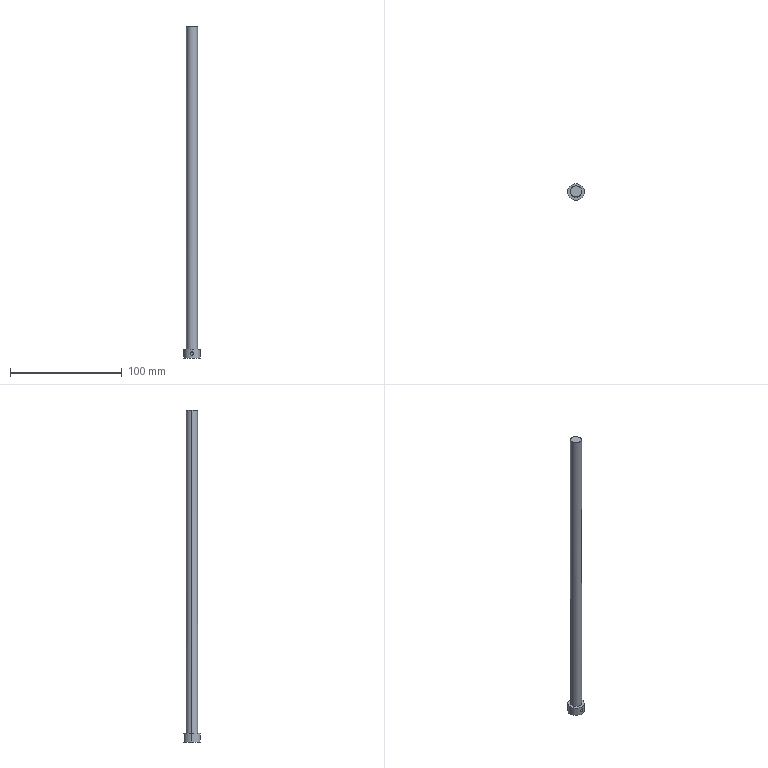Part | Creo | 1 solid | 10 faces | box 15 x 15 x 297.5 mm | volume 24082 mm3 | cylinder 6 | plane 4 | commonest cylinder face diameters 3 x2 10 x2 15 x2
STEP:
#1=CARTESIAN_POINT('',(-40.,-141.,-252.5));
#2=VERTEX_POINT('',#1);
#3=CARTESIAN_POINT('',(-50.,-141.,-252.5));
#4=VERTEX_POINT('',#3);
#5=CARTESIAN_POINT('',(-45.,-141.,-252.5));
#6=DIRECTION('',(0.,0.,-1.));
#7=DIRECTION('',(1.,0.,0.));
#8=AXIS2_PLACEMENT_3D('',#5,#6,#7);
#9=CIRCLE('',#8,5.);
#10=EDGE_CURVE('',#2,#4,#9,.T.);
#11=ORIENTED_EDGE('',*,*,#10,.T.);
#12=CARTESIAN_POINT('',(-50.,-141.,37.));
#13=VERTEX_POINT('',#12);
#14=CARTESIAN_POINT('',(-50.,-141.,37.));
#15=DIRECTION('',(0.,0.,-1.));
#16=VECTOR('',#15,289.5);
#17=LINE('',#14,#16);
#18=EDGE_CURVE('',#13,#4,#17,.T.);
#19=ORIENTED_EDGE('',*,*,#18,.F.);
#20=CARTESIAN_POINT('',(-40.,-141.,36.619));
#21=VERTEX_POINT('',#20);
#22=CARTESIAN_POINT('',(-50.,-141.,37.));
#23=CARTESIAN_POINT('',(-50.,-141.589,37.));
#24=CARTESIAN_POINT('',(-49.785,-142.862,36.992));
#25=CARTESIAN_POINT('',(-48.645,-144.641,36.949));
#26=CARTESIAN_POINT('',(-46.85,-145.786,36.88));
#27=CARTESIAN_POINT('',(-45.,-146.107,36.809));
#28=CARTESIAN_POINT('',(-43.15,-145.786,36.739));
#29=CARTESIAN_POINT('',(-41.355,-144.641,36.67));
#30=CARTESIAN_POINT('',(-40.215,-142.862,36.627));
#31=CARTESIAN_POINT('',(-40.,-141.589,36.619));
#32=CARTESIAN_POINT('',(-40.,-141.,36.619));
#33=B_SPLINE_CURVE_WITH_KNOTS('',3,(#22,#23,#24,#25,#26,#27,#28,#29,#30,#31,#32),.UNSPECIFIED.,.F.,.F.,(4,1,1,1,1,1,1,1,4),(0.,0.125,0.25,0.375,0.5,0.625,0.75,0.875,1.),.UNSPECIFIED.);
#34=EDGE_CURVE('',#13,#21,#33,.T.);
#35=ORIENTED_EDGE('',*,*,#34,.T.);
#36=CARTESIAN_POINT('',(-40.,-141.,36.619));
#37=DIRECTION('',(0.,0.,-1.));
#38=VECTOR('',#37,289.119);
#39=LINE('',#36,#38);
#40=EDGE_CURVE('',#21,#2,#39,.T.);
#41=ORIENTED_EDGE('',*,*,#40,.T.);
#42=EDGE_LOOP('',(#11,#19,#35,#41));
#43=FACE_OUTER_BOUND('',#42,.F.);
#44=CARTESIAN_POINT('',(-45.,-141.,135.));
#45=DIRECTION('',(0.,0.,-1.));
#46=DIRECTION('',(1.,0.,0.));
#47=AXIS2_PLACEMENT_3D('',#44,#45,#46);
#48=CYLINDRICAL_SURFACE('',#47,5.);
#49=ADVANCED_FACE('',(#43),#48,.T.);
#50=CARTESIAN_POINT('',(-52.5,-141.,-252.5));
#51=VERTEX_POINT('',#50);
#52=CARTESIAN_POINT('',(-37.5,-141.,-252.5));
#53=VERTEX_POINT('',#52);
#54=CARTESIAN_POINT('',(-45.,-141.,-252.5));
#55=DIRECTION('',(0.,0.,1.));
#56=DIRECTION('',(-1.,0.,0.));
#57=AXIS2_PLACEMENT_3D('',#54,#55,#56);
#58=CIRCLE('',#57,7.5);
#59=EDGE_CURVE('',#51,#53,#58,.T.);
#60=ORIENTED_EDGE('',*,*,#59,.F.);
#61=CARTESIAN_POINT('',(-45.,-141.,-252.5));
#62=DIRECTION('',(0.,0.,1.));
#63=DIRECTION('',(1.,0.,0.));
#64=AXIS2_PLACEMENT_3D('',#61,#62,#63);
#65=CIRCLE('',#64,7.5);
#66=EDGE_CURVE('',#53,#51,#65,.T.);
#67=ORIENTED_EDGE('',*,*,#66,.F.);
#68=EDGE_LOOP('',(#60,#67));
#69=FACE_OUTER_BOUND('',#68,.F.);
#70=CARTESIAN_POINT('',(-45.,-141.,-252.5));
#71=DIRECTION('',(0.,0.,-1.));
#72=DIRECTION('',(-1.,0.,0.));
#73=AXIS2_PLACEMENT_3D('',#70,#71,#72);
#74=CIRCLE('',#73,5.);
#75=EDGE_CURVE('',#4,#2,#74,.T.);
#76=ORIENTED_EDGE('',*,*,#75,.F.);
#77=ORIENTED_EDGE('',*,*,#10,.F.);
#78=EDGE_LOOP('',(#76,#77));
#79=FACE_BOUND('',#78,.F.);
#80=CARTESIAN_POINT('',(-45.,-141.,-252.5));
#81=DIRECTION('',(0.,0.,1.));
#82=DIRECTION('',(-1.,0.,0.));
#83=AXIS2_PLACEMENT_3D('',#80,#81,#82);
#84=PLANE('',#83);
#85=ADVANCED_FACE('',(#69,#79),#84,.T.);
#86=ORIENTED_EDGE('',*,*,#75,.T.);
#87=ORIENTED_EDGE('',*,*,#40,.F.);
#88=CARTESIAN_POINT('',(-40.,-141.,36.619));
#89=CARTESIAN_POINT('',(-40.,-140.411,36.619));
#90=CARTESIAN_POINT('',(-40.215,-139.138,36.627));
#91=CARTESIAN_POINT('',(-41.355,-137.359,36.67));
#92=CARTESIAN_POINT('',(-43.15,-136.214,36.739));
#93=CARTESIAN_POINT('',(-45.,-135.893,36.809));
#94=CARTESIAN_POINT('',(-46.85,-136.214,36.88));
#95=CARTESIAN_POINT('',(-48.645,-137.359,36.949));
#96=CARTESIAN_POINT('',(-49.785,-139.138,36.992));
#97=CARTESIAN_POINT('',(-50.,-140.411,37.));
#98=CARTESIAN_POINT('',(-50.,-141.,37.));
#99=B_SPLINE_CURVE_WITH_KNOTS('',3,(#88,#89,#90,#91,#92,#93,#94,#95,#96,#97,#98),.UNSPECIFIED.,.F.,.F.,(4,1,1,1,1,1,1,1,4),(0.,0.125,0.25,0.375,0.5,0.625,0.75,0.875,1.),.UNSPECIFIED.);
#100=EDGE_CURVE('',#21,#13,#99,.T.);
#101=ORIENTED_EDGE('',*,*,#100,.T.);
#102=ORIENTED_EDGE('',*,*,#18,.T.);
#103=EDGE_LOOP('',(#86,#87,#101,#102));
#104=FACE_OUTER_BOUND('',#103,.F.);
#105=CARTESIAN_POINT('',(-45.,-141.,135.));
#106=DIRECTION('',(0.,0.,-1.));
#107=DIRECTION('',(1.,0.,0.));
#108=AXIS2_PLACEMENT_3D('',#105,#106,#107);
#109=CYLINDRICAL_SURFACE('',#108,5.);
#110=ADVANCED_FACE('',(#104),#109,.T.);
#111=ORIENTED_EDGE('',*,*,#100,.F.);
#112=ORIENTED_EDGE('',*,*,#34,.F.);
#113=EDGE_LOOP('',(#111,#112));
#114=FACE_OUTER_BOUND('',#113,.F.);
#115=CARTESIAN_POINT('',(0.9569,31.474,35.055));
#116=DIRECTION('',(0.03814,0.,0.9993));
#117=DIRECTION('',(0.9993,0.,-0.03814));
#118=AXIS2_PLACEMENT_3D('',#115,#116,#117);
#119=PLANE('',#118);
#120=ADVANCED_FACE('',(#114),#119,.T.);
#121=ORIENTED_EDGE('',*,*,#59,.T.);
#122=CARTESIAN_POINT('',(-37.5,-141.,-260.5));
#123=VERTEX_POINT('',#122);
#124=CARTESIAN_POINT('',(-37.5,-141.,-260.5));
#125=DIRECTION('',(0.,0.,1.));
#126=VECTOR('',#125,8.);
#127=LINE('',#124,#126);
#128=EDGE_CURVE('',#123,#53,#127,.T.);
#129=ORIENTED_EDGE('',*,*,#128,.F.);
#130=CARTESIAN_POINT('',(-52.5,-141.,-260.5));
#131=VERTEX_POINT('',#130);
#132=CARTESIAN_POINT('',(-45.,-141.,-260.5));
#133=DIRECTION('',(0.,0.,-1.));
#134=DIRECTION('',(1.,0.,0.));
#135=AXIS2_PLACEMENT_3D('',#132,#133,#134);
#136=CIRCLE('',#135,7.5);
#137=EDGE_CURVE('',#123,#131,#136,.T.);
#138=ORIENTED_EDGE('',*,*,#137,.T.);
#139=CARTESIAN_POINT('',(-52.5,-141.,-260.5));
#140=DIRECTION('',(0.,0.,1.));
#141=VECTOR('',#140,8.);
#142=LINE('',#139,#141);
#143=EDGE_CURVE('',#131,#51,#142,.T.);
#144=ORIENTED_EDGE('',*,*,#143,.T.);
#145=EDGE_LOOP('',(#121,#129,#138,#144));
#146=FACE_OUTER_BOUND('',#145,.F.);
#147=CARTESIAN_POINT('',(-45.,-148.5,-258.));
#148=VERTEX_POINT('',#147);
#149=CARTESIAN_POINT('',(-45.,-148.5,-255.));
#150=VERTEX_POINT('',#149);
#151=CARTESIAN_POINT('',(-45.,-148.5,-258.));
#152=CARTESIAN_POINT('',(-45.205,-148.5,-258.));
#153=CARTESIAN_POINT('',(-45.583,-148.484,-257.922));
#154=CARTESIAN_POINT('',(-46.09,-148.425,-257.589));
#155=CARTESIAN_POINT('',(-46.424,-148.365,-257.085));
#156=CARTESIAN_POINT('',(-46.539,-148.34,-256.497));
#157=CARTESIAN_POINT('',(-46.422,-148.365,-255.912));
#158=CARTESIAN_POINT('',(-46.091,-148.425,-255.413));
#159=CARTESIAN_POINT('',(-45.585,-148.484,-255.078));
#160=CARTESIAN_POINT('',(-45.206,-148.5,-255.));
#161=CARTESIAN_POINT('',(-45.,-148.5,-255.));
#162=B_SPLINE_CURVE_WITH_KNOTS('',3,(#151,#152,#153,#154,#155,#156,#157,#158,#159,#160,#161),.UNSPECIFIED.,.F.,.F.,(4,1,1,1,1,1,1,1,4),(0.,0.125,0.25,0.375,0.5,0.625,0.75,0.875,1.),.UNSPECIFIED.);
#163=EDGE_CURVE('',#148,#150,#162,.T.);
#164=ORIENTED_EDGE('',*,*,#163,.F.);
#165=CARTESIAN_POINT('',(-45.,-148.5,-255.));
#166=CARTESIAN_POINT('',(-44.794,-148.5,-255.));
#167=CARTESIAN_POINT('',(-44.415,-148.484,-255.078));
#168=CARTESIAN_POINT('',(-43.907,-148.424,-255.414));
#169=CARTESIAN_POINT('',(-43.576,-148.364,-255.917));
#170=CARTESIAN_POINT('',(-43.461,-148.34,-256.506));
#171=CARTESIAN_POINT('',(-43.579,-148.365,-257.089));
#172=CARTESIAN_POINT('',(-43.908,-148.424,-257.586));
#173=CARTESIAN_POINT('',(-44.414,-148.484,-257.922));
#174=CARTESIAN_POINT('',(-44.794,-148.5,-258.));
#175=CARTESIAN_POINT('',(-45.,-148.5,-258.));
#176=B_SPLINE_CURVE_WITH_KNOTS('',3,(#165,#166,#167,#168,#169,#170,#171,#172,#173,#174,#175),.UNSPECIFIED.,.F.,.F.,(4,1,1,1,1,1,1,1,4),(0.,0.125,0.25,0.375,0.5,0.625,0.75,0.875,1.),.UNSPECIFIED.);
#177=EDGE_CURVE('',#150,#148,#176,.T.);
#178=ORIENTED_EDGE('',*,*,#177,.F.);
#179=EDGE_LOOP('',(#164,#178));
#180=FACE_BOUND('',#179,.F.);
#181=CARTESIAN_POINT('',(-45.,-141.,-260.5));
#182=DIRECTION('',(0.,0.,1.));
#183=DIRECTION('',(-1.,0.,0.));
#184=AXIS2_PLACEMENT_3D('',#181,#182,#183);
#185=CYLINDRICAL_SURFACE('',#184,7.5);
#186=ADVANCED_FACE('',(#146,#180),#185,.T.);
#187=ORIENTED_EDGE('',*,*,#163,.T.);
#188=CARTESIAN_POINT('',(-45.,-141.,-255.));
#189=VERTEX_POINT('',#188);
#190=CARTESIAN_POINT('',(-45.,-141.,-255.));
#191=DIRECTION('',(0.000000004,-1.,-0.000006083));
#192=VECTOR('',#191,7.5);
#193=LINE('',#190,#192);
#194=EDGE_CURVE('',#189,#150,#193,.T.);
#195=ORIENTED_EDGE('',*,*,#194,.F.);
#196=CARTESIAN_POINT('',(-45.,-141.,-258.));
#197=VERTEX_POINT('',#196);
#198=CARTESIAN_POINT('',(-45.,-141.,-256.5));
#199=DIRECTION('',(0.,-1.,0.));
#200=DIRECTION('',(0.,0.,1.));
#201=AXIS2_PLACEMENT_3D('',#198,#199,#200);
#202=CIRCLE('',#201,1.5);
#203=EDGE_CURVE('',#189,#197,#202,.T.);
#204=ORIENTED_EDGE('',*,*,#203,.T.);
#205=CARTESIAN_POINT('',(-45.,-141.,-258.));
#206=DIRECTION('',(0.,-1.,0.));
#207=VECTOR('',#206,7.5);
#208=LINE('',#205,#207);
#209=EDGE_CURVE('',#197,#148,#208,.T.);
#210=ORIENTED_EDGE('',*,*,#209,.T.);
#211=EDGE_LOOP('',(#187,#195,#204,#210));
#212=FACE_OUTER_BOUND('',#211,.F.);
#213=CARTESIAN_POINT('',(-45.,-141.,-256.5));
#214=DIRECTION('',(0.,-1.,0.));
#215=DIRECTION('',(0.,0.,-1.));
#216=AXIS2_PLACEMENT_3D('',#213,#214,#215);
#217=CYLINDRICAL_SURFACE('',#216,1.5);
#218=ADVANCED_FACE('',(#212),#217,.F.);
#219=ORIENTED_EDGE('',*,*,#177,.T.);
#220=ORIENTED_EDGE('',*,*,#209,.F.);
#221=CARTESIAN_POINT('',(-45.,-141.,-256.5));
#222=DIRECTION('',(0.,-1.,0.));
#223=DIRECTION('',(0.,0.,-1.));
#224=AXIS2_PLACEMENT_3D('',#221,#222,#223);
#225=CIRCLE('',#224,1.5);
#226=EDGE_CURVE('',#197,#189,#225,.T.);
#227=ORIENTED_EDGE('',*,*,#226,.T.);
#228=ORIENTED_EDGE('',*,*,#194,.T.);
#229=EDGE_LOOP('',(#219,#220,#227,#228));
#230=FACE_OUTER_BOUND('',#229,.F.);
#231=CARTESIAN_POINT('',(-45.,-141.,-256.5));
#232=DIRECTION('',(0.,-1.,0.));
#233=DIRECTION('',(0.,0.,-1.));
#234=AXIS2_PLACEMENT_3D('',#231,#232,#233);
#235=CYLINDRICAL_SURFACE('',#234,1.5);
#236=ADVANCED_FACE('',(#230),#235,.F.);
#237=ORIENTED_EDGE('',*,*,#226,.F.);
#238=ORIENTED_EDGE('',*,*,#203,.F.);
#239=EDGE_LOOP('',(#237,#238));
#240=FACE_OUTER_BOUND('',#239,.F.);
#241=CARTESIAN_POINT('',(-45.,-141.,-256.5));
#242=DIRECTION('',(0.,1.,0.));
#243=DIRECTION('',(0.,0.,1.));
#244=AXIS2_PLACEMENT_3D('',#241,#242,#243);
#245=PLANE('',#244);
#246=ADVANCED_FACE('',(#240),#245,.F.);
#247=ORIENTED_EDGE('',*,*,#66,.T.);
#248=ORIENTED_EDGE('',*,*,#143,.F.);
#249=CARTESIAN_POINT('',(-45.,-141.,-260.5));
#250=DIRECTION('',(0.,0.,-1.));
#251=DIRECTION('',(-1.,0.,0.));
#252=AXIS2_PLACEMENT_3D('',#249,#250,#251);
#253=CIRCLE('',#252,7.5);
#254=EDGE_CURVE('',#131,#123,#253,.T.);
#255=ORIENTED_EDGE('',*,*,#254,.T.);
#256=ORIENTED_EDGE('',*,*,#128,.T.);
#257=EDGE_LOOP('',(#247,#248,#255,#256));
#258=FACE_OUTER_BOUND('',#257,.F.);
#259=CARTESIAN_POINT('',(-45.,-141.,-260.5));
#260=DIRECTION('',(0.,0.,1.));
#261=DIRECTION('',(-1.,0.,0.));
#262=AXIS2_PLACEMENT_3D('',#259,#260,#261);
#263=CYLINDRICAL_SURFACE('',#262,7.5);
#264=ADVANCED_FACE('',(#258),#263,.T.);
#265=ORIENTED_EDGE('',*,*,#137,.F.);
#266=ORIENTED_EDGE('',*,*,#254,.F.);
#267=EDGE_LOOP('',(#265,#266));
#268=FACE_OUTER_BOUND('',#267,.F.);
#269=CARTESIAN_POINT('',(217.714,1.015,-260.5));
#270=DIRECTION('',(0.,0.,-1.));
#271=DIRECTION('',(1.,0.,0.));
#272=AXIS2_PLACEMENT_3D('',#269,#270,#271);
#273=PLANE('',#272);
#274=ADVANCED_FACE('',(#268),#273,.T.);
#275=CLOSED_SHELL('',(#49,#85,#110,#120,#186,#218,#236,#246,#264,#274));
#276=MANIFOLD_SOLID_BREP('',#275);
#277=(LENGTH_UNIT()NAMED_UNIT(*)SI_UNIT(.MILLI.,.METRE.));
#278=UNCERTAINTY_MEASURE_WITH_UNIT(LENGTH_MEASURE(0.02982),#277,'','');
#279=(NAMED_UNIT(*)PLANE_ANGLE_UNIT()SI_UNIT($,.RADIAN.));
#280=PLANE_ANGLE_MEASURE_WITH_UNIT(PLANE_ANGLE_MEASURE(0.01745),#279);
#281=(CONVERSION_BASED_UNIT('DEGREE',#280)NAMED_UNIT(*)PLANE_ANGLE_UNIT());
#282=(NAMED_UNIT(*)SI_UNIT($,.STERADIAN.)SOLID_ANGLE_UNIT());
#283=(GEOMETRIC_REPRESENTATION_CONTEXT(3)GLOBAL_UNCERTAINTY_ASSIGNED_CONTEXT((#278))GLOBAL_UNIT_ASSIGNED_CONTEXT((#277,#281,#282))REPRESENTATION_CONTEXT('',''));
#284=ADVANCED_BREP_SHAPE_REPRESENTATION('',(#276),#283);